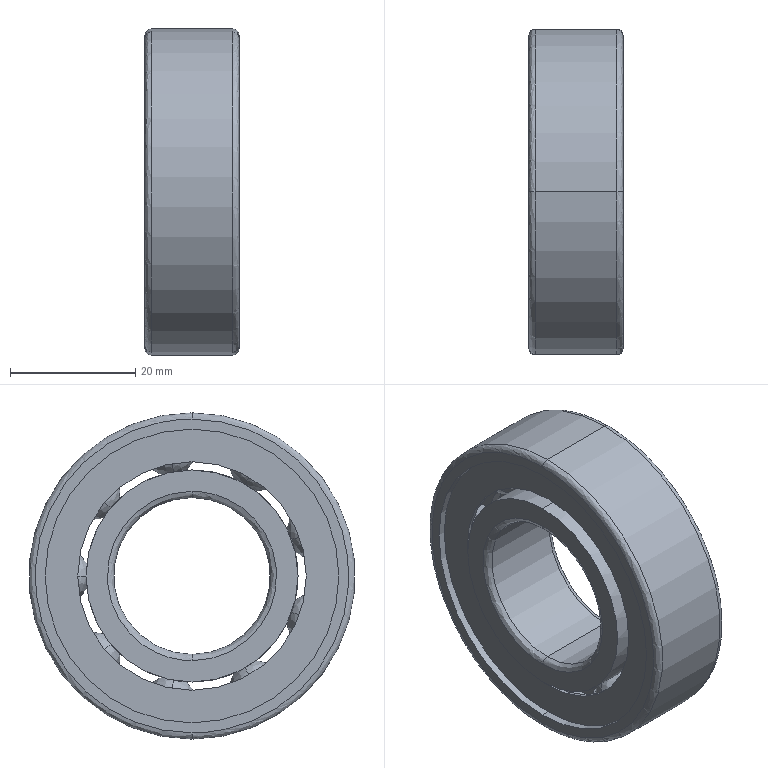Part | STEP file | 1 solid | 160 faces | box 15 x 52 x 52 mm | volume 14938 mm3 | spline 110 | plane 26 | cylinder 24 | commonest cylinder face diameters 46.8 x8 33.8 x4 36.42 x4 25 x2 38.117 x2 42.483 x2